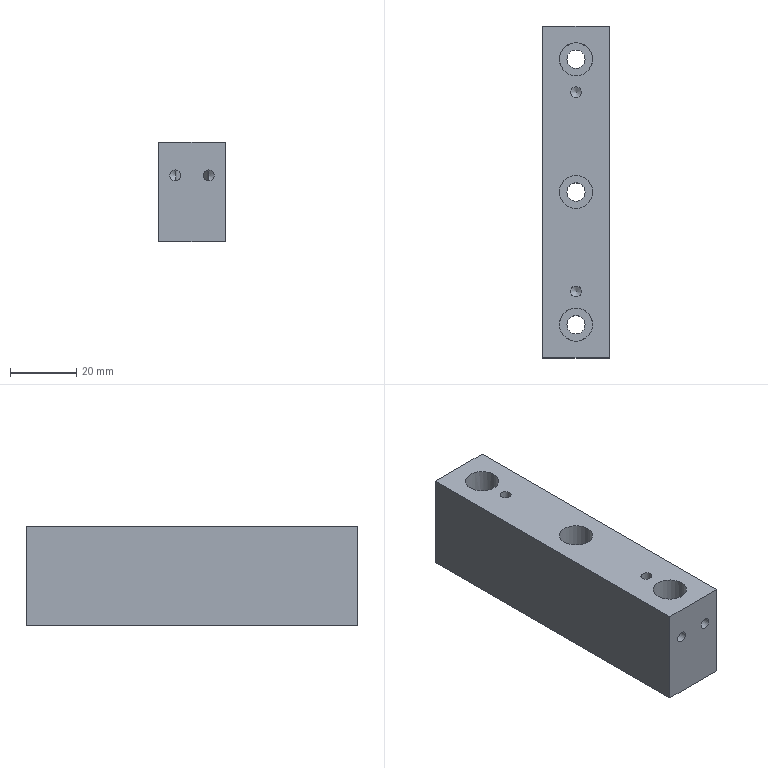Part | NX | 1 solid | 29 faces | box 20 x 100 x 30 mm | volume 54087 mm3 | cylinder 14 | plane 9 | cone 6 | commonest cylinder face diameters 3.3 x8 5.5 x3 10 x3
STEP:
#1=CARTESIAN_POINT('',(10.,-50.,0.));
#2=VERTEX_POINT('',#1);
#3=CARTESIAN_POINT('',(10.,50.,0.));
#4=VERTEX_POINT('',#3);
#5=CARTESIAN_POINT('',(10.,50.,0.));
#6=DIRECTION('',(0.,1.,0.));
#7=VECTOR('',#6,1000.);
#8=LINE('',#5,#7);
#9=EDGE_CURVE('',#2,#4,#8,.T.);
#10=ORIENTED_EDGE('',*,*,#9,.T.);
#11=CARTESIAN_POINT('',(10.,50.,30.));
#12=VERTEX_POINT('',#11);
#13=CARTESIAN_POINT('',(10.,50.,30.));
#14=DIRECTION('',(0.,0.,-1.));
#15=VECTOR('',#14,1000.);
#16=LINE('',#13,#15);
#17=EDGE_CURVE('',#12,#4,#16,.T.);
#18=ORIENTED_EDGE('',*,*,#17,.F.);
#19=CARTESIAN_POINT('',(10.,-50.,30.));
#20=VERTEX_POINT('',#19);
#21=CARTESIAN_POINT('',(10.,50.,30.));
#22=DIRECTION('',(0.,1.,0.));
#23=VECTOR('',#22,1000.);
#24=LINE('',#21,#23);
#25=EDGE_CURVE('',#20,#12,#24,.T.);
#26=ORIENTED_EDGE('',*,*,#25,.F.);
#27=CARTESIAN_POINT('',(10.,-50.,30.));
#28=DIRECTION('',(0.,0.,-1.));
#29=VECTOR('',#28,1000.);
#30=LINE('',#27,#29);
#31=EDGE_CURVE('',#20,#2,#30,.T.);
#32=ORIENTED_EDGE('',*,*,#31,.T.);
#33=EDGE_LOOP('',(#10,#18,#26,#32));
#34=FACE_BOUND('',#33,.T.);
#35=CARTESIAN_POINT('',(10.,50.,30.));
#36=DIRECTION('',(-1.,0.,0.));
#37=DIRECTION('',(0.,-1.,0.));
#38=AXIS2_PLACEMENT_3D('',#35,#36,#37);
#39=PLANE('',#38);
#40=ADVANCED_FACE('',(#34),#39,.F.);
#41=CARTESIAN_POINT('',(-5.,50.,21.65));
#42=VERTEX_POINT('',#41);
#43=CARTESIAN_POINT('',(-5.,50.,20.));
#44=DIRECTION('',(0.,1.,0.));
#45=DIRECTION('',(0.,0.,1.));
#46=AXIS2_PLACEMENT_3D('',#43,#44,#45);
#47=CIRCLE('',#46,1.65);
#48=EDGE_CURVE('',#42,#42,#47,.T.);
#49=ORIENTED_EDGE('',*,*,#48,.F.);
#50=EDGE_LOOP('',(#49));
#51=FACE_BOUND('',#50,.T.);
#52=CARTESIAN_POINT('',(5.,50.,21.65));
#53=VERTEX_POINT('',#52);
#54=CARTESIAN_POINT('',(5.,50.,20.));
#55=DIRECTION('',(0.,1.,0.));
#56=DIRECTION('',(0.,0.,1.));
#57=AXIS2_PLACEMENT_3D('',#54,#55,#56);
#58=CIRCLE('',#57,1.65);
#59=EDGE_CURVE('',#53,#53,#58,.T.);
#60=ORIENTED_EDGE('',*,*,#59,.F.);
#61=EDGE_LOOP('',(#60));
#62=FACE_BOUND('',#61,.T.);
#63=CARTESIAN_POINT('',(-10.,50.,0.));
#64=VERTEX_POINT('',#63);
#65=CARTESIAN_POINT('',(-10.,50.,0.));
#66=DIRECTION('',(-1.,0.,0.));
#67=VECTOR('',#66,1000.);
#68=LINE('',#65,#67);
#69=EDGE_CURVE('',#4,#64,#68,.T.);
#70=ORIENTED_EDGE('',*,*,#69,.T.);
#71=CARTESIAN_POINT('',(-10.,50.,30.));
#72=VERTEX_POINT('',#71);
#73=CARTESIAN_POINT('',(-10.,50.,30.));
#74=DIRECTION('',(0.,0.,-1.));
#75=VECTOR('',#74,1000.);
#76=LINE('',#73,#75);
#77=EDGE_CURVE('',#72,#64,#76,.T.);
#78=ORIENTED_EDGE('',*,*,#77,.F.);
#79=CARTESIAN_POINT('',(-10.,50.,30.));
#80=DIRECTION('',(-1.,0.,0.));
#81=VECTOR('',#80,1000.);
#82=LINE('',#79,#81);
#83=EDGE_CURVE('',#12,#72,#82,.T.);
#84=ORIENTED_EDGE('',*,*,#83,.F.);
#85=ORIENTED_EDGE('',*,*,#17,.T.);
#86=EDGE_LOOP('',(#70,#78,#84,#85));
#87=FACE_BOUND('',#86,.T.);
#88=CARTESIAN_POINT('',(-10.,50.,30.));
#89=DIRECTION('',(0.,-1.,0.));
#90=DIRECTION('',(0.,0.,-1.));
#91=AXIS2_PLACEMENT_3D('',#88,#89,#90);
#92=PLANE('',#91);
#93=ADVANCED_FACE('',(#51,#62,#87),#92,.F.);
#94=CARTESIAN_POINT('',(-10.,-50.,0.));
#95=VERTEX_POINT('',#94);
#96=CARTESIAN_POINT('',(-10.,50.,0.));
#97=DIRECTION('',(0.,-1.,0.));
#98=VECTOR('',#97,1000.);
#99=LINE('',#96,#98);
#100=EDGE_CURVE('',#64,#95,#99,.T.);
#101=ORIENTED_EDGE('',*,*,#100,.T.);
#102=CARTESIAN_POINT('',(-10.,-50.,30.));
#103=VERTEX_POINT('',#102);
#104=CARTESIAN_POINT('',(-10.,-50.,30.));
#105=DIRECTION('',(0.,0.,-1.));
#106=VECTOR('',#105,1000.);
#107=LINE('',#104,#106);
#108=EDGE_CURVE('',#103,#95,#107,.T.);
#109=ORIENTED_EDGE('',*,*,#108,.F.);
#110=CARTESIAN_POINT('',(-10.,50.,30.));
#111=DIRECTION('',(0.,-1.,0.));
#112=VECTOR('',#111,1000.);
#113=LINE('',#110,#112);
#114=EDGE_CURVE('',#72,#103,#113,.T.);
#115=ORIENTED_EDGE('',*,*,#114,.F.);
#116=ORIENTED_EDGE('',*,*,#77,.T.);
#117=EDGE_LOOP('',(#101,#109,#115,#116));
#118=FACE_BOUND('',#117,.T.);
#119=CARTESIAN_POINT('',(-10.,50.,30.));
#120=DIRECTION('',(1.,0.,0.));
#121=DIRECTION('',(0.,1.,0.));
#122=AXIS2_PLACEMENT_3D('',#119,#120,#121);
#123=PLANE('',#122);
#124=ADVANCED_FACE('',(#118),#123,.F.);
#125=CARTESIAN_POINT('',(-5.,-50.,18.35));
#126=VERTEX_POINT('',#125);
#127=CARTESIAN_POINT('',(-5.,-50.,20.));
#128=DIRECTION('',(0.,-1.,0.));
#129=DIRECTION('',(0.,0.,-1.));
#130=AXIS2_PLACEMENT_3D('',#127,#128,#129);
#131=CIRCLE('',#130,1.65);
#132=EDGE_CURVE('',#126,#126,#131,.T.);
#133=ORIENTED_EDGE('',*,*,#132,.F.);
#134=EDGE_LOOP('',(#133));
#135=FACE_BOUND('',#134,.T.);
#136=CARTESIAN_POINT('',(5.,-50.,18.35));
#137=VERTEX_POINT('',#136);
#138=CARTESIAN_POINT('',(5.,-50.,20.));
#139=DIRECTION('',(0.,-1.,0.));
#140=DIRECTION('',(0.,0.,-1.));
#141=AXIS2_PLACEMENT_3D('',#138,#139,#140);
#142=CIRCLE('',#141,1.65);
#143=EDGE_CURVE('',#137,#137,#142,.T.);
#144=ORIENTED_EDGE('',*,*,#143,.F.);
#145=EDGE_LOOP('',(#144));
#146=FACE_BOUND('',#145,.T.);
#147=CARTESIAN_POINT('',(-10.,-50.,0.));
#148=DIRECTION('',(1.,0.,0.));
#149=VECTOR('',#148,1000.);
#150=LINE('',#147,#149);
#151=EDGE_CURVE('',#95,#2,#150,.T.);
#152=ORIENTED_EDGE('',*,*,#151,.T.);
#153=ORIENTED_EDGE('',*,*,#31,.F.);
#154=CARTESIAN_POINT('',(-10.,-50.,30.));
#155=DIRECTION('',(1.,0.,0.));
#156=VECTOR('',#155,1000.);
#157=LINE('',#154,#156);
#158=EDGE_CURVE('',#103,#20,#157,.T.);
#159=ORIENTED_EDGE('',*,*,#158,.F.);
#160=ORIENTED_EDGE('',*,*,#108,.T.);
#161=EDGE_LOOP('',(#152,#153,#159,#160));
#162=FACE_BOUND('',#161,.T.);
#163=CARTESIAN_POINT('',(-10.,-50.,30.));
#164=DIRECTION('',(0.,1.,0.));
#165=DIRECTION('',(0.,0.,1.));
#166=AXIS2_PLACEMENT_3D('',#163,#164,#165);
#167=PLANE('',#166);
#168=ADVANCED_FACE('',(#135,#146,#162),#167,.F.);
#169=CARTESIAN_POINT('',(1.65,30.,30.));
#170=VERTEX_POINT('',#169);
#171=CARTESIAN_POINT('',(0.,30.,30.));
#172=DIRECTION('',(0.,0.,1.));
#173=DIRECTION('',(1.,0.,0.));
#174=AXIS2_PLACEMENT_3D('',#171,#172,#173);
#175=CIRCLE('',#174,1.65);
#176=EDGE_CURVE('',#170,#170,#175,.T.);
#177=ORIENTED_EDGE('',*,*,#176,.F.);
#178=EDGE_LOOP('',(#177));
#179=FACE_BOUND('',#178,.T.);
#180=CARTESIAN_POINT('',(1.65,-30.,30.));
#181=VERTEX_POINT('',#180);
#182=CARTESIAN_POINT('',(0.,-30.,30.));
#183=DIRECTION('',(0.,0.,1.));
#184=DIRECTION('',(1.,0.,0.));
#185=AXIS2_PLACEMENT_3D('',#182,#183,#184);
#186=CIRCLE('',#185,1.65);
#187=EDGE_CURVE('',#181,#181,#186,.T.);
#188=ORIENTED_EDGE('',*,*,#187,.F.);
#189=EDGE_LOOP('',(#188));
#190=FACE_BOUND('',#189,.T.);
#191=CARTESIAN_POINT('',(5.,40.,30.));
#192=VERTEX_POINT('',#191);
#193=CARTESIAN_POINT('',(0.,40.,30.));
#194=DIRECTION('',(0.,0.,1.));
#195=DIRECTION('',(1.,0.,0.));
#196=AXIS2_PLACEMENT_3D('',#193,#194,#195);
#197=CIRCLE('',#196,5.);
#198=EDGE_CURVE('',#192,#192,#197,.T.);
#199=ORIENTED_EDGE('',*,*,#198,.F.);
#200=EDGE_LOOP('',(#199));
#201=FACE_BOUND('',#200,.T.);
#202=CARTESIAN_POINT('',(5.,0.,30.));
#203=VERTEX_POINT('',#202);
#204=CARTESIAN_POINT('',(0.,0.,30.));
#205=DIRECTION('',(0.,0.,1.));
#206=DIRECTION('',(1.,0.,0.));
#207=AXIS2_PLACEMENT_3D('',#204,#205,#206);
#208=CIRCLE('',#207,5.);
#209=EDGE_CURVE('',#203,#203,#208,.T.);
#210=ORIENTED_EDGE('',*,*,#209,.F.);
#211=EDGE_LOOP('',(#210));
#212=FACE_BOUND('',#211,.T.);
#213=CARTESIAN_POINT('',(5.,-40.,30.));
#214=VERTEX_POINT('',#213);
#215=CARTESIAN_POINT('',(0.,-40.,30.));
#216=DIRECTION('',(0.,0.,1.));
#217=DIRECTION('',(1.,0.,0.));
#218=AXIS2_PLACEMENT_3D('',#215,#216,#217);
#219=CIRCLE('',#218,5.);
#220=EDGE_CURVE('',#214,#214,#219,.T.);
#221=ORIENTED_EDGE('',*,*,#220,.F.);
#222=EDGE_LOOP('',(#221));
#223=FACE_BOUND('',#222,.T.);
#224=ORIENTED_EDGE('',*,*,#25,.T.);
#225=ORIENTED_EDGE('',*,*,#83,.T.);
#226=ORIENTED_EDGE('',*,*,#114,.T.);
#227=ORIENTED_EDGE('',*,*,#158,.T.);
#228=EDGE_LOOP('',(#224,#225,#226,#227));
#229=FACE_BOUND('',#228,.T.);
#230=CARTESIAN_POINT('',(0.,0.,30.));
#231=DIRECTION('',(0.,0.,1.));
#232=DIRECTION('',(1.,0.,0.));
#233=AXIS2_PLACEMENT_3D('',#230,#231,#232);
#234=PLANE('',#233);
#235=ADVANCED_FACE('',(#179,#190,#201,#212,#223,#229),#234,.T.);
#236=CARTESIAN_POINT('',(2.75,40.,0.));
#237=VERTEX_POINT('',#236);
#238=CARTESIAN_POINT('',(0.,40.,0.));
#239=DIRECTION('',(0.,0.,1.));
#240=DIRECTION('',(1.,0.,0.));
#241=AXIS2_PLACEMENT_3D('',#238,#239,#240);
#242=CIRCLE('',#241,2.75);
#243=EDGE_CURVE('',#237,#237,#242,.T.);
#244=ORIENTED_EDGE('',*,*,#243,.T.);
#245=EDGE_LOOP('',(#244));
#246=FACE_BOUND('',#245,.T.);
#247=CARTESIAN_POINT('',(2.75,0.,0.));
#248=VERTEX_POINT('',#247);
#249=CARTESIAN_POINT('',(0.,0.,0.));
#250=DIRECTION('',(0.,0.,1.));
#251=DIRECTION('',(1.,0.,0.));
#252=AXIS2_PLACEMENT_3D('',#249,#250,#251);
#253=CIRCLE('',#252,2.75);
#254=EDGE_CURVE('',#248,#248,#253,.T.);
#255=ORIENTED_EDGE('',*,*,#254,.T.);
#256=EDGE_LOOP('',(#255));
#257=FACE_BOUND('',#256,.T.);
#258=CARTESIAN_POINT('',(2.75,-40.,0.));
#259=VERTEX_POINT('',#258);
#260=CARTESIAN_POINT('',(0.,-40.,0.));
#261=DIRECTION('',(0.,0.,1.));
#262=DIRECTION('',(1.,0.,0.));
#263=AXIS2_PLACEMENT_3D('',#260,#261,#262);
#264=CIRCLE('',#263,2.75);
#265=EDGE_CURVE('',#259,#259,#264,.T.);
#266=ORIENTED_EDGE('',*,*,#265,.T.);
#267=EDGE_LOOP('',(#266));
#268=FACE_BOUND('',#267,.T.);
#269=ORIENTED_EDGE('',*,*,#9,.F.);
#270=ORIENTED_EDGE('',*,*,#151,.F.);
#271=ORIENTED_EDGE('',*,*,#100,.F.);
#272=ORIENTED_EDGE('',*,*,#69,.F.);
#273=EDGE_LOOP('',(#269,#270,#271,#272));
#274=FACE_BOUND('',#273,.T.);
#275=CARTESIAN_POINT('',(0.,0.,0.));
#276=DIRECTION('',(0.,0.,1.));
#277=DIRECTION('',(1.,0.,0.));
#278=AXIS2_PLACEMENT_3D('',#275,#276,#277);
#279=PLANE('',#278);
#280=ADVANCED_FACE('',(#246,#257,#268,#274),#279,.F.);
#281=ORIENTED_EDGE('',*,*,#265,.F.);
#282=EDGE_LOOP('',(#281));
#283=FACE_BOUND('',#282,.T.);
#284=CARTESIAN_POINT('',(2.75,-40.,10.));
#285=VERTEX_POINT('',#284);
#286=CARTESIAN_POINT('',(0.,-40.,10.));
#287=DIRECTION('',(0.,0.,1.));
#288=DIRECTION('',(1.,0.,0.));
#289=AXIS2_PLACEMENT_3D('',#286,#287,#288);
#290=CIRCLE('',#289,2.75);
#291=EDGE_CURVE('',#285,#285,#290,.T.);
#292=ORIENTED_EDGE('',*,*,#291,.T.);
#293=EDGE_LOOP('',(#292));
#294=FACE_BOUND('',#293,.T.);
#295=CARTESIAN_POINT('',(0.,-40.,30.));
#296=DIRECTION('',(0.,0.,1.));
#297=DIRECTION('',(1.,0.,0.));
#298=AXIS2_PLACEMENT_3D('',#295,#296,#297);
#299=CYLINDRICAL_SURFACE('',#298,2.75);
#300=ADVANCED_FACE('',(#283,#294),#299,.F.);
#301=ORIENTED_EDGE('',*,*,#291,.F.);
#302=EDGE_LOOP('',(#301));
#303=FACE_BOUND('',#302,.T.);
#304=CARTESIAN_POINT('',(5.,-40.,10.));
#305=VERTEX_POINT('',#304);
#306=CARTESIAN_POINT('',(0.,-40.,10.));
#307=DIRECTION('',(0.,0.,1.));
#308=DIRECTION('',(1.,0.,0.));
#309=AXIS2_PLACEMENT_3D('',#306,#307,#308);
#310=CIRCLE('',#309,5.);
#311=EDGE_CURVE('',#305,#305,#310,.T.);
#312=ORIENTED_EDGE('',*,*,#311,.T.);
#313=EDGE_LOOP('',(#312));
#314=FACE_BOUND('',#313,.T.);
#315=CARTESIAN_POINT('',(2.75,-40.,10.));
#316=DIRECTION('',(0.,0.,-1.));
#317=DIRECTION('',(-1.,0.,0.));
#318=AXIS2_PLACEMENT_3D('',#315,#316,#317);
#319=PLANE('',#318);
#320=ADVANCED_FACE('',(#303,#314),#319,.F.);
#321=CARTESIAN_POINT('',(-4.999,-39.9,21.65));
#322=VERTEX_POINT('',#321);
#323=CARTESIAN_POINT('',(-4.999,-39.9,18.35));
#324=VERTEX_POINT('',#323);
#325=CARTESIAN_POINT('',(-4.999,-39.9,21.65));
#326=CARTESIAN_POINT('',(-4.996,-39.736,21.377));
#327=CARTESIAN_POINT('',(-4.977,-39.48,20.965));
#328=CARTESIAN_POINT('',(-4.935,-39.18,20.428));
#329=CARTESIAN_POINT('',(-4.872,-38.867,19.99));
#330=CARTESIAN_POINT('',(-4.937,-39.189,19.563));
#331=CARTESIAN_POINT('',(-4.977,-39.483,19.028));
#332=CARTESIAN_POINT('',(-4.996,-39.737,18.621));
#333=CARTESIAN_POINT('',(-4.999,-39.9,18.35));
#334=B_SPLINE_CURVE_WITH_KNOTS('',3,(#325,#326,#327,#328,#329,#330,#331,#332,#333),.UNSPECIFIED.,.F.,.F.,(4,1,1,1,1,1,4),(0.0001928,0.001148,0.001626,0.002103,0.002581,0.003059,0.004014),.UNSPECIFIED.);
#335=EDGE_CURVE('',#322,#324,#334,.T.);
#336=ORIENTED_EDGE('',*,*,#335,.T.);
#337=CARTESIAN_POINT('',(-4.999,-39.9,18.35));
#338=CARTESIAN_POINT('',(-5.008,-40.325,18.35));
#339=CARTESIAN_POINT('',(-4.917,-41.161,18.344));
#340=CARTESIAN_POINT('',(-4.473,-42.36,18.403));
#341=CARTESIAN_POINT('',(-3.729,-43.388,18.77));
#342=CARTESIAN_POINT('',(-3.161,-43.873,19.996));
#343=CARTESIAN_POINT('',(-3.727,-43.39,21.229));
#344=CARTESIAN_POINT('',(-4.47,-42.364,21.596));
#345=CARTESIAN_POINT('',(-4.914,-41.173,21.656));
#346=CARTESIAN_POINT('',(-5.008,-40.325,21.65));
#347=CARTESIAN_POINT('',(-4.999,-39.9,21.65));
#348=B_SPLINE_CURVE_WITH_KNOTS('',3,(#337,#338,#339,#340,#341,#342,#343,#344,#345,#346,#347),.UNSPECIFIED.,.F.,.F.,(4,1,1,1,1,1,1,1,4),(0.,0.001258,0.002516,0.003774,0.005031,0.006289,0.007547,0.008805,0.01006),.UNSPECIFIED.);
#349=EDGE_CURVE('',#324,#322,#348,.T.);
#350=ORIENTED_EDGE('',*,*,#349,.T.);
#351=EDGE_LOOP('',(#336,#350));
#352=FACE_BOUND('',#351,.T.);
#353=CARTESIAN_POINT('',(4.999,-39.9,18.35));
#354=VERTEX_POINT('',#353);
#355=CARTESIAN_POINT('',(4.999,-39.9,21.65));
#356=VERTEX_POINT('',#355);
#357=CARTESIAN_POINT('',(4.999,-39.9,18.35));
#358=CARTESIAN_POINT('',(4.996,-39.736,18.623));
#359=CARTESIAN_POINT('',(4.977,-39.48,19.035));
#360=CARTESIAN_POINT('',(4.935,-39.18,19.572));
#361=CARTESIAN_POINT('',(4.872,-38.867,20.01));
#362=CARTESIAN_POINT('',(4.937,-39.189,20.437));
#363=CARTESIAN_POINT('',(4.977,-39.483,20.972));
#364=CARTESIAN_POINT('',(4.996,-39.737,21.379));
#365=CARTESIAN_POINT('',(4.999,-39.9,21.65));
#366=B_SPLINE_CURVE_WITH_KNOTS('',3,(#357,#358,#359,#360,#361,#362,#363,#364,#365),.UNSPECIFIED.,.F.,.F.,(4,1,1,1,1,1,4),(0.0001928,0.001148,0.001626,0.002103,0.002581,0.003059,0.004014),.UNSPECIFIED.);
#367=EDGE_CURVE('',#354,#356,#366,.T.);
#368=ORIENTED_EDGE('',*,*,#367,.T.);
#369=CARTESIAN_POINT('',(4.999,-39.9,21.65));
#370=CARTESIAN_POINT('',(5.008,-40.325,21.65));
#371=CARTESIAN_POINT('',(4.917,-41.161,21.656));
#372=CARTESIAN_POINT('',(4.473,-42.36,21.597));
#373=CARTESIAN_POINT('',(3.729,-43.388,21.23));
#374=CARTESIAN_POINT('',(3.161,-43.873,20.004));
#375=CARTESIAN_POINT('',(3.727,-43.39,18.771));
#376=CARTESIAN_POINT('',(4.47,-42.364,18.404));
#377=CARTESIAN_POINT('',(4.914,-41.173,18.344));
#378=CARTESIAN_POINT('',(5.008,-40.325,18.35));
#379=CARTESIAN_POINT('',(4.999,-39.9,18.35));
#380=B_SPLINE_CURVE_WITH_KNOTS('',3,(#369,#370,#371,#372,#373,#374,#375,#376,#377,#378,#379),.UNSPECIFIED.,.F.,.F.,(4,1,1,1,1,1,1,1,4),(0.,0.001258,0.002516,0.003774,0.005031,0.006289,0.007547,0.008805,0.01006),.UNSPECIFIED.);
#381=EDGE_CURVE('',#356,#354,#380,.T.);
#382=ORIENTED_EDGE('',*,*,#381,.T.);
#383=EDGE_LOOP('',(#368,#382));
#384=FACE_BOUND('',#383,.T.);
#385=ORIENTED_EDGE('',*,*,#311,.F.);
#386=EDGE_LOOP('',(#385));
#387=FACE_BOUND('',#386,.T.);
#388=ORIENTED_EDGE('',*,*,#220,.T.);
#389=EDGE_LOOP('',(#388));
#390=FACE_BOUND('',#389,.T.);
#391=CARTESIAN_POINT('',(0.,-40.,30.));
#392=DIRECTION('',(0.,0.,1.));
#393=DIRECTION('',(1.,0.,0.));
#394=AXIS2_PLACEMENT_3D('',#391,#392,#393);
#395=CYLINDRICAL_SURFACE('',#394,5.);
#396=ADVANCED_FACE('',(#352,#384,#387,#390),#395,.F.);
#397=ORIENTED_EDGE('',*,*,#254,.F.);
#398=EDGE_LOOP('',(#397));
#399=FACE_BOUND('',#398,.T.);
#400=CARTESIAN_POINT('',(2.75,0.,10.));
#401=VERTEX_POINT('',#400);
#402=CARTESIAN_POINT('',(0.,0.,10.));
#403=DIRECTION('',(0.,0.,1.));
#404=DIRECTION('',(1.,0.,0.));
#405=AXIS2_PLACEMENT_3D('',#402,#403,#404);
#406=CIRCLE('',#405,2.75);
#407=EDGE_CURVE('',#401,#401,#406,.T.);
#408=ORIENTED_EDGE('',*,*,#407,.T.);
#409=EDGE_LOOP('',(#408));
#410=FACE_BOUND('',#409,.T.);
#411=CARTESIAN_POINT('',(0.,0.,30.));
#412=DIRECTION('',(0.,0.,1.));
#413=DIRECTION('',(1.,0.,0.));
#414=AXIS2_PLACEMENT_3D('',#411,#412,#413);
#415=CYLINDRICAL_SURFACE('',#414,2.75);
#416=ADVANCED_FACE('',(#399,#410),#415,.F.);
#417=ORIENTED_EDGE('',*,*,#407,.F.);
#418=EDGE_LOOP('',(#417));
#419=FACE_BOUND('',#418,.T.);
#420=CARTESIAN_POINT('',(5.,0.,10.));
#421=VERTEX_POINT('',#420);
#422=CARTESIAN_POINT('',(0.,0.,10.));
#423=DIRECTION('',(0.,0.,1.));
#424=DIRECTION('',(1.,0.,0.));
#425=AXIS2_PLACEMENT_3D('',#422,#423,#424);
#426=CIRCLE('',#425,5.);
#427=EDGE_CURVE('',#421,#421,#426,.T.);
#428=ORIENTED_EDGE('',*,*,#427,.T.);
#429=EDGE_LOOP('',(#428));
#430=FACE_BOUND('',#429,.T.);
#431=CARTESIAN_POINT('',(2.75,0.,10.));
#432=DIRECTION('',(0.,0.,-1.));
#433=DIRECTION('',(-1.,0.,0.));
#434=AXIS2_PLACEMENT_3D('',#431,#432,#433);
#435=PLANE('',#434);
#436=ADVANCED_FACE('',(#419,#430),#435,.F.);
#437=ORIENTED_EDGE('',*,*,#427,.F.);
#438=EDGE_LOOP('',(#437));
#439=FACE_BOUND('',#438,.T.);
#440=ORIENTED_EDGE('',*,*,#209,.T.);
#441=EDGE_LOOP('',(#440));
#442=FACE_BOUND('',#441,.T.);
#443=CARTESIAN_POINT('',(0.,0.,30.));
#444=DIRECTION('',(0.,0.,1.));
#445=DIRECTION('',(1.,0.,0.));
#446=AXIS2_PLACEMENT_3D('',#443,#444,#445);
#447=CYLINDRICAL_SURFACE('',#446,5.);
#448=ADVANCED_FACE('',(#439,#442),#447,.F.);
#449=ORIENTED_EDGE('',*,*,#243,.F.);
#450=EDGE_LOOP('',(#449));
#451=FACE_BOUND('',#450,.T.);
#452=CARTESIAN_POINT('',(2.75,40.,10.));
#453=VERTEX_POINT('',#452);
#454=CARTESIAN_POINT('',(0.,40.,10.));
#455=DIRECTION('',(0.,0.,1.));
#456=DIRECTION('',(1.,0.,0.));
#457=AXIS2_PLACEMENT_3D('',#454,#455,#456);
#458=CIRCLE('',#457,2.75);
#459=EDGE_CURVE('',#453,#453,#458,.T.);
#460=ORIENTED_EDGE('',*,*,#459,.T.);
#461=EDGE_LOOP('',(#460));
#462=FACE_BOUND('',#461,.T.);
#463=CARTESIAN_POINT('',(0.,40.,30.));
#464=DIRECTION('',(0.,0.,1.));
#465=DIRECTION('',(1.,0.,0.));
#466=AXIS2_PLACEMENT_3D('',#463,#464,#465);
#467=CYLINDRICAL_SURFACE('',#466,2.75);
#468=ADVANCED_FACE('',(#451,#462),#467,.F.);
#469=ORIENTED_EDGE('',*,*,#459,.F.);
#470=EDGE_LOOP('',(#469));
#471=FACE_BOUND('',#470,.T.);
#472=CARTESIAN_POINT('',(5.,40.,10.));
#473=VERTEX_POINT('',#472);
#474=CARTESIAN_POINT('',(0.,40.,10.));
#475=DIRECTION('',(0.,0.,1.));
#476=DIRECTION('',(1.,0.,0.));
#477=AXIS2_PLACEMENT_3D('',#474,#475,#476);
#478=CIRCLE('',#477,5.);
#479=EDGE_CURVE('',#473,#473,#478,.T.);
#480=ORIENTED_EDGE('',*,*,#479,.T.);
#481=EDGE_LOOP('',(#480));
#482=FACE_BOUND('',#481,.T.);
#483=CARTESIAN_POINT('',(2.75,40.,10.));
#484=DIRECTION('',(0.,0.,-1.));
#485=DIRECTION('',(-1.,0.,0.));
#486=AXIS2_PLACEMENT_3D('',#483,#484,#485);
#487=PLANE('',#486);
#488=ADVANCED_FACE('',(#471,#482),#487,.F.);
#489=CARTESIAN_POINT('',(-4.999,39.9,18.35));
#490=VERTEX_POINT('',#489);
#491=CARTESIAN_POINT('',(-4.999,39.9,21.65));
#492=VERTEX_POINT('',#491);
#493=CARTESIAN_POINT('',(-4.999,39.9,18.35));
#494=CARTESIAN_POINT('',(-4.996,39.736,18.623));
#495=CARTESIAN_POINT('',(-4.977,39.48,19.035));
#496=CARTESIAN_POINT('',(-4.935,39.18,19.572));
#497=CARTESIAN_POINT('',(-4.872,38.867,20.01));
#498=CARTESIAN_POINT('',(-4.937,39.189,20.437));
#499=CARTESIAN_POINT('',(-4.977,39.483,20.972));
#500=CARTESIAN_POINT('',(-4.996,39.737,21.379));
#501=CARTESIAN_POINT('',(-4.999,39.9,21.65));
#502=B_SPLINE_CURVE_WITH_KNOTS('',3,(#493,#494,#495,#496,#497,#498,#499,#500,#501),.UNSPECIFIED.,.F.,.F.,(4,1,1,1,1,1,4),(0.0001928,0.001148,0.001626,0.002103,0.002581,0.003059,0.004014),.UNSPECIFIED.);
#503=EDGE_CURVE('',#490,#492,#502,.T.);
#504=ORIENTED_EDGE('',*,*,#503,.T.);
#505=CARTESIAN_POINT('',(-4.999,39.9,21.65));
#506=CARTESIAN_POINT('',(-5.008,40.325,21.65));
#507=CARTESIAN_POINT('',(-4.917,41.161,21.656));
#508=CARTESIAN_POINT('',(-4.473,42.36,21.597));
#509=CARTESIAN_POINT('',(-3.729,43.388,21.23));
#510=CARTESIAN_POINT('',(-3.161,43.873,20.004));
#511=CARTESIAN_POINT('',(-3.727,43.39,18.771));
#512=CARTESIAN_POINT('',(-4.47,42.364,18.404));
#513=CARTESIAN_POINT('',(-4.914,41.173,18.344));
#514=CARTESIAN_POINT('',(-5.008,40.325,18.35));
#515=CARTESIAN_POINT('',(-4.999,39.9,18.35));
#516=B_SPLINE_CURVE_WITH_KNOTS('',3,(#505,#506,#507,#508,#509,#510,#511,#512,#513,#514,#515),.UNSPECIFIED.,.F.,.F.,(4,1,1,1,1,1,1,1,4),(0.,0.001258,0.002516,0.003774,0.005031,0.006289,0.007547,0.008805,0.01006),.UNSPECIFIED.);
#517=EDGE_CURVE('',#492,#490,#516,.T.);
#518=ORIENTED_EDGE('',*,*,#517,.T.);
#519=EDGE_LOOP('',(#504,#518));
#520=FACE_BOUND('',#519,.T.);
#521=CARTESIAN_POINT('',(4.999,39.9,21.65));
#522=VERTEX_POINT('',#521);
#523=CARTESIAN_POINT('',(4.999,39.9,18.35));
#524=VERTEX_POINT('',#523);
#525=CARTESIAN_POINT('',(4.999,39.9,21.65));
#526=CARTESIAN_POINT('',(4.996,39.736,21.377));
#527=CARTESIAN_POINT('',(4.977,39.48,20.965));
#528=CARTESIAN_POINT('',(4.935,39.18,20.428));
#529=CARTESIAN_POINT('',(4.872,38.867,19.99));
#530=CARTESIAN_POINT('',(4.937,39.189,19.563));
#531=CARTESIAN_POINT('',(4.977,39.483,19.028));
#532=CARTESIAN_POINT('',(4.996,39.737,18.621));
#533=CARTESIAN_POINT('',(4.999,39.9,18.35));
#534=B_SPLINE_CURVE_WITH_KNOTS('',3,(#525,#526,#527,#528,#529,#530,#531,#532,#533),.UNSPECIFIED.,.F.,.F.,(4,1,1,1,1,1,4),(0.0001928,0.001148,0.001626,0.002103,0.002581,0.003059,0.004014),.UNSPECIFIED.);
#535=EDGE_CURVE('',#522,#524,#534,.T.);
#536=ORIENTED_EDGE('',*,*,#535,.T.);
#537=CARTESIAN_POINT('',(4.999,39.9,18.35));
#538=CARTESIAN_POINT('',(5.008,40.325,18.35));
#539=CARTESIAN_POINT('',(4.917,41.161,18.344));
#540=CARTESIAN_POINT('',(4.473,42.36,18.403));
#541=CARTESIAN_POINT('',(3.729,43.388,18.77));
#542=CARTESIAN_POINT('',(3.161,43.873,19.996));
#543=CARTESIAN_POINT('',(3.727,43.39,21.229));
#544=CARTESIAN_POINT('',(4.47,42.364,21.596));
#545=CARTESIAN_POINT('',(4.914,41.173,21.656));
#546=CARTESIAN_POINT('',(5.008,40.325,21.65));
#547=CARTESIAN_POINT('',(4.999,39.9,21.65));
#548=B_SPLINE_CURVE_WITH_KNOTS('',3,(#537,#538,#539,#540,#541,#542,#543,#544,#545,#546,#547),.UNSPECIFIED.,.F.,.F.,(4,1,1,1,1,1,1,1,4),(0.,0.001258,0.002516,0.003774,0.005031,0.006289,0.007547,0.008805,0.01006),.UNSPECIFIED.);
#549=EDGE_CURVE('',#524,#522,#548,.T.);
#550=ORIENTED_EDGE('',*,*,#549,.T.);
#551=EDGE_LOOP('',(#536,#550));
#552=FACE_BOUND('',#551,.T.);
#553=ORIENTED_EDGE('',*,*,#479,.F.);
#554=EDGE_LOOP('',(#553));
#555=FACE_BOUND('',#554,.T.);
#556=ORIENTED_EDGE('',*,*,#198,.T.);
#557=EDGE_LOOP('',(#556));
#558=FACE_BOUND('',#557,.T.);
#559=CARTESIAN_POINT('',(0.,40.,30.));
#560=DIRECTION('',(0.,0.,1.));
#561=DIRECTION('',(1.,0.,0.));
#562=AXIS2_PLACEMENT_3D('',#559,#560,#561);
#563=CYLINDRICAL_SURFACE('',#562,5.);
#564=ADVANCED_FACE('',(#520,#552,#555,#558),#563,.F.);
#565=CARTESIAN_POINT('',(0.,-30.,18.909));
#566=VERTEX_POINT('',#565);
#567=VERTEX_LOOP('',#566);
#568=FACE_BOUND('',#567,.T.);
#569=CARTESIAN_POINT('',(1.65,-30.,19.9));
#570=VERTEX_POINT('',#569);
#571=CARTESIAN_POINT('',(0.,-30.,19.9));
#572=DIRECTION('',(0.,0.,1.));
#573=DIRECTION('',(1.,0.,0.));
#574=AXIS2_PLACEMENT_3D('',#571,#572,#573);
#575=CIRCLE('',#574,1.65);
#576=EDGE_CURVE('',#570,#570,#575,.T.);
#577=ORIENTED_EDGE('',*,*,#576,.T.);
#578=EDGE_LOOP('',(#577));
#579=FACE_BOUND('',#578,.T.);
#580=CARTESIAN_POINT('',(0.,-30.,19.9));
#581=DIRECTION('',(0.,0.,1.));
#582=DIRECTION('',(1.,0.,0.));
#583=AXIS2_PLACEMENT_3D('',#580,#581,#582);
#584=CONICAL_SURFACE('',#583,1.65,1.03);
#585=ADVANCED_FACE('',(#568,#579),#584,.F.);
#586=ORIENTED_EDGE('',*,*,#576,.F.);
#587=EDGE_LOOP('',(#586));
#588=FACE_BOUND('',#587,.T.);
#589=ORIENTED_EDGE('',*,*,#187,.T.);
#590=EDGE_LOOP('',(#589));
#591=FACE_BOUND('',#590,.T.);
#592=CARTESIAN_POINT('',(0.,-30.,30.));
#593=DIRECTION('',(0.,0.,1.));
#594=DIRECTION('',(1.,0.,0.));
#595=AXIS2_PLACEMENT_3D('',#592,#593,#594);
#596=CYLINDRICAL_SURFACE('',#595,1.65);
#597=ADVANCED_FACE('',(#588,#591),#596,.F.);
#598=CARTESIAN_POINT('',(0.,30.,18.909));
#599=VERTEX_POINT('',#598);
#600=VERTEX_LOOP('',#599);
#601=FACE_BOUND('',#600,.T.);
#602=CARTESIAN_POINT('',(1.65,30.,19.9));
#603=VERTEX_POINT('',#602);
#604=CARTESIAN_POINT('',(0.,30.,19.9));
#605=DIRECTION('',(0.,0.,1.));
#606=DIRECTION('',(1.,0.,0.));
#607=AXIS2_PLACEMENT_3D('',#604,#605,#606);
#608=CIRCLE('',#607,1.65);
#609=EDGE_CURVE('',#603,#603,#608,.T.);
#610=ORIENTED_EDGE('',*,*,#609,.T.);
#611=EDGE_LOOP('',(#610));
#612=FACE_BOUND('',#611,.T.);
#613=CARTESIAN_POINT('',(0.,30.,19.9));
#614=DIRECTION('',(0.,0.,1.));
#615=DIRECTION('',(1.,0.,0.));
#616=AXIS2_PLACEMENT_3D('',#613,#614,#615);
#617=CONICAL_SURFACE('',#616,1.65,1.03);
#618=ADVANCED_FACE('',(#601,#612),#617,.F.);
#619=ORIENTED_EDGE('',*,*,#609,.F.);
#620=EDGE_LOOP('',(#619));
#621=FACE_BOUND('',#620,.T.);
#622=ORIENTED_EDGE('',*,*,#176,.T.);
#623=EDGE_LOOP('',(#622));
#624=FACE_BOUND('',#623,.T.);
#625=CARTESIAN_POINT('',(0.,30.,30.));
#626=DIRECTION('',(0.,0.,1.));
#627=DIRECTION('',(1.,0.,0.));
#628=AXIS2_PLACEMENT_3D('',#625,#626,#627);
#629=CYLINDRICAL_SURFACE('',#628,1.65);
#630=ADVANCED_FACE('',(#621,#624),#629,.F.);
#631=ORIENTED_EDGE('',*,*,#143,.T.);
#632=EDGE_LOOP('',(#631));
#633=FACE_BOUND('',#632,.T.);
#634=CARTESIAN_POINT('',(5.,-39.9,20.));
#635=DIRECTION('',(0.,-1.,0.));
#636=DIRECTION('',(0.,0.,-1.));
#637=AXIS2_PLACEMENT_3D('',#634,#635,#636);
#638=CIRCLE('',#637,1.65);
#639=EDGE_CURVE('',#354,#356,#638,.T.);
#640=ORIENTED_EDGE('',*,*,#639,.F.);
#641=ORIENTED_EDGE('',*,*,#381,.F.);
#642=EDGE_LOOP('',(#640,#641));
#643=FACE_BOUND('',#642,.T.);
#644=CARTESIAN_POINT('',(5.,-50.,20.));
#645=DIRECTION('',(0.,-1.,0.));
#646=DIRECTION('',(0.,0.,-1.));
#647=AXIS2_PLACEMENT_3D('',#644,#645,#646);
#648=CYLINDRICAL_SURFACE('',#647,1.65);
#649=ADVANCED_FACE('',(#633,#643),#648,.F.);
#650=CARTESIAN_POINT('',(5.,-38.909,20.));
#651=VERTEX_POINT('',#650);
#652=VERTEX_LOOP('',#651);
#653=FACE_BOUND('',#652,.T.);
#654=ORIENTED_EDGE('',*,*,#639,.T.);
#655=ORIENTED_EDGE('',*,*,#367,.F.);
#656=EDGE_LOOP('',(#654,#655));
#657=FACE_BOUND('',#656,.T.);
#658=CARTESIAN_POINT('',(5.,-39.9,20.));
#659=DIRECTION('',(0.,-1.,0.));
#660=DIRECTION('',(0.,0.,-1.));
#661=AXIS2_PLACEMENT_3D('',#658,#659,#660);
#662=CONICAL_SURFACE('',#661,1.65,1.03);
#663=ADVANCED_FACE('',(#653,#657),#662,.F.);
#664=ORIENTED_EDGE('',*,*,#132,.T.);
#665=EDGE_LOOP('',(#664));
#666=FACE_BOUND('',#665,.T.);
#667=CARTESIAN_POINT('',(-5.,-39.9,20.));
#668=DIRECTION('',(0.,-1.,0.));
#669=DIRECTION('',(0.,0.,-1.));
#670=AXIS2_PLACEMENT_3D('',#667,#668,#669);
#671=CIRCLE('',#670,1.65);
#672=EDGE_CURVE('',#322,#324,#671,.T.);
#673=ORIENTED_EDGE('',*,*,#672,.F.);
#674=ORIENTED_EDGE('',*,*,#349,.F.);
#675=EDGE_LOOP('',(#673,#674));
#676=FACE_BOUND('',#675,.T.);
#677=CARTESIAN_POINT('',(-5.,-50.,20.));
#678=DIRECTION('',(0.,-1.,0.));
#679=DIRECTION('',(0.,0.,-1.));
#680=AXIS2_PLACEMENT_3D('',#677,#678,#679);
#681=CYLINDRICAL_SURFACE('',#680,1.65);
#682=ADVANCED_FACE('',(#666,#676),#681,.F.);
#683=CARTESIAN_POINT('',(-5.,-38.909,20.));
#684=VERTEX_POINT('',#683);
#685=VERTEX_LOOP('',#684);
#686=FACE_BOUND('',#685,.T.);
#687=ORIENTED_EDGE('',*,*,#672,.T.);
#688=ORIENTED_EDGE('',*,*,#335,.F.);
#689=EDGE_LOOP('',(#687,#688));
#690=FACE_BOUND('',#689,.T.);
#691=CARTESIAN_POINT('',(-5.,-39.9,20.));
#692=DIRECTION('',(0.,-1.,0.));
#693=DIRECTION('',(0.,0.,-1.));
#694=AXIS2_PLACEMENT_3D('',#691,#692,#693);
#695=CONICAL_SURFACE('',#694,1.65,1.03);
#696=ADVANCED_FACE('',(#686,#690),#695,.F.);
#697=ORIENTED_EDGE('',*,*,#59,.T.);
#698=EDGE_LOOP('',(#697));
#699=FACE_BOUND('',#698,.T.);
#700=CARTESIAN_POINT('',(5.,39.9,20.));
#701=DIRECTION('',(0.,1.,0.));
#702=DIRECTION('',(0.,0.,1.));
#703=AXIS2_PLACEMENT_3D('',#700,#701,#702);
#704=CIRCLE('',#703,1.65);
#705=EDGE_CURVE('',#522,#524,#704,.T.);
#706=ORIENTED_EDGE('',*,*,#705,.F.);
#707=ORIENTED_EDGE('',*,*,#549,.F.);
#708=EDGE_LOOP('',(#706,#707));
#709=FACE_BOUND('',#708,.T.);
#710=CARTESIAN_POINT('',(5.,50.,20.));
#711=DIRECTION('',(0.,1.,0.));
#712=DIRECTION('',(0.,0.,1.));
#713=AXIS2_PLACEMENT_3D('',#710,#711,#712);
#714=CYLINDRICAL_SURFACE('',#713,1.65);
#715=ADVANCED_FACE('',(#699,#709),#714,.F.);
#716=CARTESIAN_POINT('',(5.,38.909,20.));
#717=VERTEX_POINT('',#716);
#718=VERTEX_LOOP('',#717);
#719=FACE_BOUND('',#718,.T.);
#720=ORIENTED_EDGE('',*,*,#705,.T.);
#721=ORIENTED_EDGE('',*,*,#535,.F.);
#722=EDGE_LOOP('',(#720,#721));
#723=FACE_BOUND('',#722,.T.);
#724=CARTESIAN_POINT('',(5.,39.9,20.));
#725=DIRECTION('',(0.,1.,0.));
#726=DIRECTION('',(0.,0.,1.));
#727=AXIS2_PLACEMENT_3D('',#724,#725,#726);
#728=CONICAL_SURFACE('',#727,1.65,1.03);
#729=ADVANCED_FACE('',(#719,#723),#728,.F.);
#730=ORIENTED_EDGE('',*,*,#48,.T.);
#731=EDGE_LOOP('',(#730));
#732=FACE_BOUND('',#731,.T.);
#733=CARTESIAN_POINT('',(-5.,39.9,20.));
#734=DIRECTION('',(0.,1.,0.));
#735=DIRECTION('',(0.,0.,1.));
#736=AXIS2_PLACEMENT_3D('',#733,#734,#735);
#737=CIRCLE('',#736,1.65);
#738=EDGE_CURVE('',#490,#492,#737,.T.);
#739=ORIENTED_EDGE('',*,*,#738,.F.);
#740=ORIENTED_EDGE('',*,*,#517,.F.);
#741=EDGE_LOOP('',(#739,#740));
#742=FACE_BOUND('',#741,.T.);
#743=CARTESIAN_POINT('',(-5.,50.,20.));
#744=DIRECTION('',(0.,1.,0.));
#745=DIRECTION('',(0.,0.,1.));
#746=AXIS2_PLACEMENT_3D('',#743,#744,#745);
#747=CYLINDRICAL_SURFACE('',#746,1.65);
#748=ADVANCED_FACE('',(#732,#742),#747,.F.);
#749=CARTESIAN_POINT('',(-5.,38.909,20.));
#750=VERTEX_POINT('',#749);
#751=VERTEX_LOOP('',#750);
#752=FACE_BOUND('',#751,.T.);
#753=ORIENTED_EDGE('',*,*,#738,.T.);
#754=ORIENTED_EDGE('',*,*,#503,.F.);
#755=EDGE_LOOP('',(#753,#754));
#756=FACE_BOUND('',#755,.T.);
#757=CARTESIAN_POINT('',(-5.,39.9,20.));
#758=DIRECTION('',(0.,1.,0.));
#759=DIRECTION('',(0.,0.,1.));
#760=AXIS2_PLACEMENT_3D('',#757,#758,#759);
#761=CONICAL_SURFACE('',#760,1.65,1.03);
#762=ADVANCED_FACE('',(#752,#756),#761,.F.);
#763=CLOSED_SHELL('',(#40,#93,#124,#168,#235,#280,#300,#320,#396,#416,#436,#448,#468,#488,#564,#585,#597,#618,#630,#649,#663,#682,#696,#715,#729,#748,#762));
#764=MANIFOLD_SOLID_BREP('',#763);
#765=(LENGTH_UNIT()NAMED_UNIT(*)SI_UNIT(.MILLI.,.METRE.));
#766=UNCERTAINTY_MEASURE_WITH_UNIT(LENGTH_MEASURE(0.0508),#765,'','');
#767=(NAMED_UNIT(*)PLANE_ANGLE_UNIT()SI_UNIT($,.RADIAN.));
#768=(NAMED_UNIT(*)SI_UNIT($,.STERADIAN.)SOLID_ANGLE_UNIT());
#769=(GEOMETRIC_REPRESENTATION_CONTEXT(3)GLOBAL_UNCERTAINTY_ASSIGNED_CONTEXT((#766))GLOBAL_UNIT_ASSIGNED_CONTEXT((#765,#767,#768))REPRESENTATION_CONTEXT('',''));
#770=ADVANCED_BREP_SHAPE_REPRESENTATION('',(#764),#769);